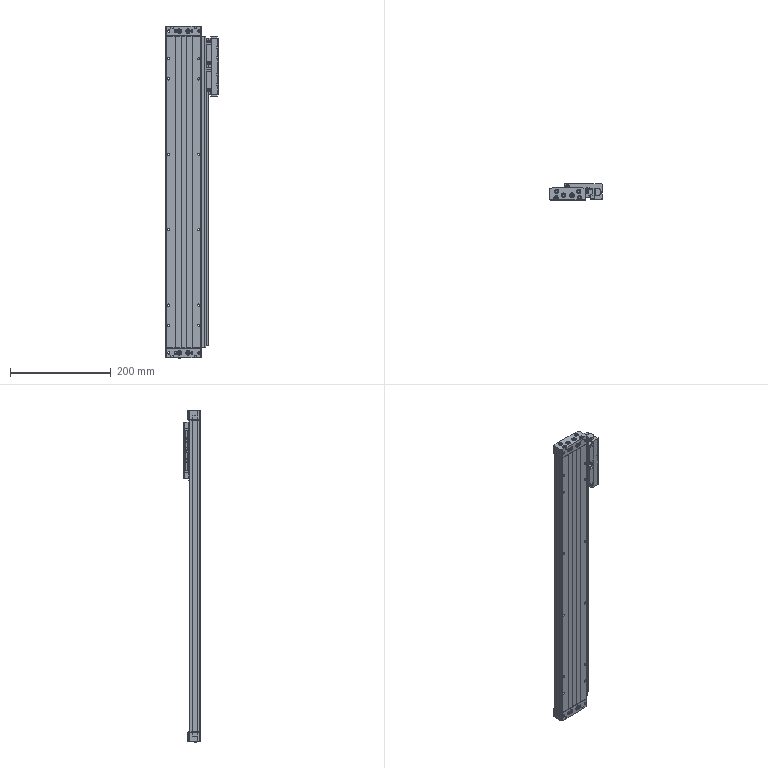Part | SolidWorks | features AEMSimFeature 1 | 13 solids | 1650 faces | box 105 x 32 x 660 mm | volume 1112378 mm3 | plane 619 | cylinder 600 | cone 263 | spline 168 | commonest cylinder face diameters 1 x67 0.4 x64 8 x54 3 x52 2 x36 9 x34